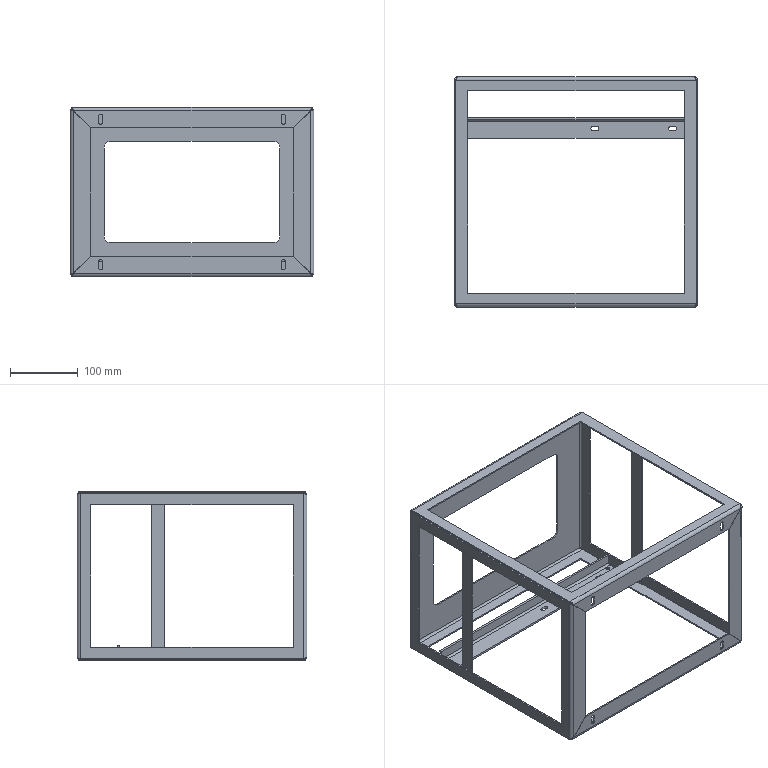Part | STEP file | Ice maker bracket V1.201001 | 4 solids | 182 faces | box 360 x 340 x 250 mm | volume 395832 mm3 | plane 102 | cylinder 64 | spline 16 | commonest cylinder face diameters 6 x47 10 x8 2.5 x4 20 x4 12 x1